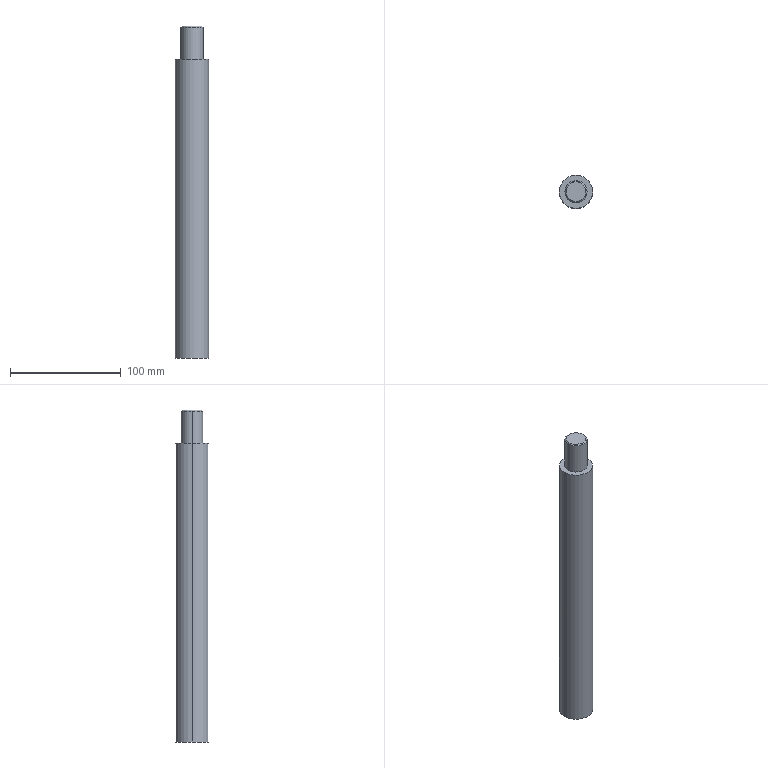Part | STEP file | Telescopic Rod 2 | 1 solid | 9 faces | box 30 x 30 x 300 mm | volume 200246 mm3 | cylinder 4 | plane 3 | cone 2 | commonest cylinder face diameters 20 x2 30 x2
STEP:
#1=CARTESIAN_POINT('',(-15.,0.,270.));
#2=VERTEX_POINT('',#1);
#3=CARTESIAN_POINT('',(15.,0.,270.));
#4=VERTEX_POINT('',#3);
#5=CARTESIAN_POINT('',(0.,0.,270.));
#6=DIRECTION('',(0.,0.,-1.));
#7=DIRECTION('',(-1.,0.,0.));
#8=AXIS2_PLACEMENT_3D('',#5,#6,#7);
#9=CIRCLE('',#8,15.);
#10=EDGE_CURVE('',#2,#4,#9,.T.);
#11=ORIENTED_EDGE('',*,*,#10,.T.);
#12=CARTESIAN_POINT('',(15.,0.,0.));
#13=VERTEX_POINT('',#12);
#14=CARTESIAN_POINT('',(15.,0.,300.));
#15=DIRECTION('',(0.,0.,-1.));
#16=VECTOR('',#15,1000.);
#17=LINE('',#14,#16);
#18=EDGE_CURVE('',#4,#13,#17,.T.);
#19=ORIENTED_EDGE('',*,*,#18,.T.);
#20=CARTESIAN_POINT('',(-15.,0.,0.));
#21=VERTEX_POINT('',#20);
#22=CARTESIAN_POINT('',(0.,0.,0.));
#23=DIRECTION('',(0.,0.,1.));
#24=DIRECTION('',(-1.,0.,0.));
#25=AXIS2_PLACEMENT_3D('',#22,#23,#24);
#26=CIRCLE('',#25,15.);
#27=EDGE_CURVE('',#13,#21,#26,.T.);
#28=ORIENTED_EDGE('',*,*,#27,.T.);
#29=CARTESIAN_POINT('',(-15.,0.,300.));
#30=DIRECTION('',(0.,0.,-1.));
#31=VECTOR('',#30,1000.);
#32=LINE('',#29,#31);
#33=EDGE_CURVE('',#2,#21,#32,.T.);
#34=ORIENTED_EDGE('',*,*,#33,.F.);
#35=EDGE_LOOP('',(#11,#19,#28,#34));
#36=FACE_OUTER_BOUND('',#35,.T.);
#37=CARTESIAN_POINT('',(0.,0.,300.));
#38=DIRECTION('',(0.,0.,-1.));
#39=DIRECTION('',(-1.,0.,0.));
#40=AXIS2_PLACEMENT_3D('',#37,#38,#39);
#41=CYLINDRICAL_SURFACE('',#40,15.);
#42=ADVANCED_FACE('',(#36),#41,.T.);
#43=CARTESIAN_POINT('',(-10.,0.,270.));
#44=VERTEX_POINT('',#43);
#45=CARTESIAN_POINT('',(10.,0.,270.));
#46=VERTEX_POINT('',#45);
#47=CARTESIAN_POINT('',(0.,0.,270.));
#48=DIRECTION('',(0.,0.,-1.));
#49=DIRECTION('',(1.,0.,0.));
#50=AXIS2_PLACEMENT_3D('',#47,#48,#49);
#51=CIRCLE('',#50,10.);
#52=EDGE_CURVE('',#44,#46,#51,.T.);
#53=ORIENTED_EDGE('',*,*,#52,.F.);
#54=CARTESIAN_POINT('',(-10.,0.,299.));
#55=VERTEX_POINT('',#54);
#56=CARTESIAN_POINT('',(-10.,0.,270.));
#57=DIRECTION('',(0.,0.,1.));
#58=VECTOR('',#57,1000.);
#59=LINE('',#56,#58);
#60=EDGE_CURVE('',#44,#55,#59,.T.);
#61=ORIENTED_EDGE('',*,*,#60,.T.);
#62=CARTESIAN_POINT('',(10.,0.,299.));
#63=VERTEX_POINT('',#62);
#64=CARTESIAN_POINT('',(0.,0.,299.));
#65=DIRECTION('',(0.,0.,-1.));
#66=DIRECTION('',(1.,0.,0.));
#67=AXIS2_PLACEMENT_3D('',#64,#65,#66);
#68=CIRCLE('',#67,10.);
#69=EDGE_CURVE('',#55,#63,#68,.T.);
#70=ORIENTED_EDGE('',*,*,#69,.T.);
#71=CARTESIAN_POINT('',(10.,0.,270.));
#72=DIRECTION('',(0.,0.,1.));
#73=VECTOR('',#72,1000.);
#74=LINE('',#71,#73);
#75=EDGE_CURVE('',#46,#63,#74,.T.);
#76=ORIENTED_EDGE('',*,*,#75,.F.);
#77=EDGE_LOOP('',(#53,#61,#70,#76));
#78=FACE_OUTER_BOUND('',#77,.T.);
#79=CARTESIAN_POINT('',(0.,0.,270.));
#80=DIRECTION('',(0.,0.,1.));
#81=DIRECTION('',(1.,0.,0.));
#82=AXIS2_PLACEMENT_3D('',#79,#80,#81);
#83=CYLINDRICAL_SURFACE('',#82,10.);
#84=ADVANCED_FACE('',(#78),#83,.T.);
#85=CARTESIAN_POINT('',(-9.,0.,300.));
#86=VERTEX_POINT('',#85);
#87=CARTESIAN_POINT('',(9.,0.,300.));
#88=VERTEX_POINT('',#87);
#89=CARTESIAN_POINT('',(0.,0.,300.));
#90=DIRECTION('',(0.,0.,-1.));
#91=DIRECTION('',(-1.,0.,0.));
#92=AXIS2_PLACEMENT_3D('',#89,#90,#91);
#93=CIRCLE('',#92,9.);
#94=EDGE_CURVE('',#86,#88,#93,.T.);
#95=ORIENTED_EDGE('',*,*,#94,.T.);
#96=CARTESIAN_POINT('',(10.,0.,299.));
#97=DIRECTION('',(0.7071,0.,-0.7071));
#98=VECTOR('',#97,1000.);
#99=LINE('',#96,#98);
#100=EDGE_CURVE('',#88,#63,#99,.T.);
#101=ORIENTED_EDGE('',*,*,#100,.T.);
#102=ORIENTED_EDGE('',*,*,#69,.F.);
#103=CARTESIAN_POINT('',(-10.,0.,299.));
#104=DIRECTION('',(-0.7071,0.,-0.7071));
#105=VECTOR('',#104,1000.);
#106=LINE('',#103,#105);
#107=EDGE_CURVE('',#86,#55,#106,.T.);
#108=ORIENTED_EDGE('',*,*,#107,.F.);
#109=EDGE_LOOP('',(#95,#101,#102,#108));
#110=FACE_OUTER_BOUND('',#109,.T.);
#111=CARTESIAN_POINT('',(0.,0.,299.));
#112=DIRECTION('',(0.,0.,-1.));
#113=DIRECTION('',(-1.,0.,0.));
#114=AXIS2_PLACEMENT_3D('',#111,#112,#113);
#115=CONICAL_SURFACE('',#114,10.,0.7854);
#116=ADVANCED_FACE('',(#110),#115,.T.);
#117=ORIENTED_EDGE('',*,*,#18,.F.);
#118=CARTESIAN_POINT('',(0.,0.,270.));
#119=DIRECTION('',(0.,0.,-1.));
#120=DIRECTION('',(-1.,0.,0.));
#121=AXIS2_PLACEMENT_3D('',#118,#119,#120);
#122=CIRCLE('',#121,15.);
#123=EDGE_CURVE('',#4,#2,#122,.T.);
#124=ORIENTED_EDGE('',*,*,#123,.T.);
#125=ORIENTED_EDGE('',*,*,#33,.T.);
#126=CARTESIAN_POINT('',(0.,0.,0.));
#127=DIRECTION('',(0.,0.,1.));
#128=DIRECTION('',(-1.,0.,0.));
#129=AXIS2_PLACEMENT_3D('',#126,#127,#128);
#130=CIRCLE('',#129,15.);
#131=EDGE_CURVE('',#21,#13,#130,.T.);
#132=ORIENTED_EDGE('',*,*,#131,.T.);
#133=EDGE_LOOP('',(#117,#124,#125,#132));
#134=FACE_OUTER_BOUND('',#133,.T.);
#135=CARTESIAN_POINT('',(0.,0.,300.));
#136=DIRECTION('',(0.,0.,-1.));
#137=DIRECTION('',(-1.,0.,0.));
#138=AXIS2_PLACEMENT_3D('',#135,#136,#137);
#139=CYLINDRICAL_SURFACE('',#138,15.);
#140=ADVANCED_FACE('',(#134),#139,.T.);
#141=ORIENTED_EDGE('',*,*,#131,.F.);
#142=ORIENTED_EDGE('',*,*,#27,.F.);
#143=EDGE_LOOP('',(#141,#142));
#144=FACE_OUTER_BOUND('',#143,.T.);
#145=CARTESIAN_POINT('',(0.,0.,0.));
#146=DIRECTION('',(0.,0.,1.));
#147=DIRECTION('',(1.,0.,0.));
#148=AXIS2_PLACEMENT_3D('',#145,#146,#147);
#149=PLANE('',#148);
#150=ADVANCED_FACE('',(#144),#149,.F.);
#151=ORIENTED_EDGE('',*,*,#10,.F.);
#152=ORIENTED_EDGE('',*,*,#123,.F.);
#153=EDGE_LOOP('',(#151,#152));
#154=FACE_OUTER_BOUND('',#153,.T.);
#155=CARTESIAN_POINT('',(0.,0.,270.));
#156=DIRECTION('',(0.,0.,-1.));
#157=DIRECTION('',(1.,0.,0.));
#158=AXIS2_PLACEMENT_3D('',#155,#156,#157);
#159=CIRCLE('',#158,10.);
#160=EDGE_CURVE('',#46,#44,#159,.T.);
#161=ORIENTED_EDGE('',*,*,#160,.T.);
#162=ORIENTED_EDGE('',*,*,#52,.T.);
#163=EDGE_LOOP('',(#161,#162));
#164=FACE_BOUND('',#163,.T.);
#165=CARTESIAN_POINT('',(0.,0.,270.));
#166=DIRECTION('',(0.,0.,1.));
#167=DIRECTION('',(1.,0.,0.));
#168=AXIS2_PLACEMENT_3D('',#165,#166,#167);
#169=PLANE('',#168);
#170=ADVANCED_FACE('',(#154,#164),#169,.T.);
#171=ORIENTED_EDGE('',*,*,#60,.F.);
#172=ORIENTED_EDGE('',*,*,#160,.F.);
#173=ORIENTED_EDGE('',*,*,#75,.T.);
#174=CARTESIAN_POINT('',(0.,0.,299.));
#175=DIRECTION('',(0.,0.,-1.));
#176=DIRECTION('',(1.,0.,0.));
#177=AXIS2_PLACEMENT_3D('',#174,#175,#176);
#178=CIRCLE('',#177,10.);
#179=EDGE_CURVE('',#63,#55,#178,.T.);
#180=ORIENTED_EDGE('',*,*,#179,.T.);
#181=EDGE_LOOP('',(#171,#172,#173,#180));
#182=FACE_OUTER_BOUND('',#181,.T.);
#183=CARTESIAN_POINT('',(0.,0.,270.));
#184=DIRECTION('',(0.,0.,1.));
#185=DIRECTION('',(1.,0.,0.));
#186=AXIS2_PLACEMENT_3D('',#183,#184,#185);
#187=CYLINDRICAL_SURFACE('',#186,10.);
#188=ADVANCED_FACE('',(#182),#187,.T.);
#189=ORIENTED_EDGE('',*,*,#100,.F.);
#190=CARTESIAN_POINT('',(0.,0.,300.));
#191=DIRECTION('',(0.,0.,-1.));
#192=DIRECTION('',(-1.,0.,0.));
#193=AXIS2_PLACEMENT_3D('',#190,#191,#192);
#194=CIRCLE('',#193,9.);
#195=EDGE_CURVE('',#88,#86,#194,.T.);
#196=ORIENTED_EDGE('',*,*,#195,.T.);
#197=ORIENTED_EDGE('',*,*,#107,.T.);
#198=ORIENTED_EDGE('',*,*,#179,.F.);
#199=EDGE_LOOP('',(#189,#196,#197,#198));
#200=FACE_OUTER_BOUND('',#199,.T.);
#201=CARTESIAN_POINT('',(0.,0.,299.));
#202=DIRECTION('',(0.,0.,-1.));
#203=DIRECTION('',(-1.,0.,0.));
#204=AXIS2_PLACEMENT_3D('',#201,#202,#203);
#205=CONICAL_SURFACE('',#204,10.,0.7854);
#206=ADVANCED_FACE('',(#200),#205,.T.);
#207=ORIENTED_EDGE('',*,*,#94,.F.);
#208=ORIENTED_EDGE('',*,*,#195,.F.);
#209=EDGE_LOOP('',(#207,#208));
#210=FACE_OUTER_BOUND('',#209,.T.);
#211=CARTESIAN_POINT('',(0.,0.,300.));
#212=DIRECTION('',(0.,0.,1.));
#213=DIRECTION('',(1.,0.,0.));
#214=AXIS2_PLACEMENT_3D('',#211,#212,#213);
#215=PLANE('',#214);
#216=ADVANCED_FACE('',(#210),#215,.T.);
#217=CLOSED_SHELL('',(#42,#84,#116,#140,#150,#170,#188,#206,#216));
#218=MANIFOLD_SOLID_BREP('',#217);
#219=CARTESIAN_POINT('',(0.,0.,0.));
#220=DIRECTION('',(0.,0.,1.));
#221=DIRECTION('',(1.,0.,0.));
#222=AXIS2_PLACEMENT_3D('',#219,#220,#221);
#223=(LENGTH_UNIT()NAMED_UNIT(*)SI_UNIT(.MILLI.,.METRE.));
#224=UNCERTAINTY_MEASURE_WITH_UNIT(LENGTH_MEASURE(0.00001),#223,'','');
#225=(NAMED_UNIT(*)PLANE_ANGLE_UNIT()SI_UNIT($,.RADIAN.));
#226=(NAMED_UNIT(*)SI_UNIT($,.STERADIAN.)SOLID_ANGLE_UNIT());
#227=(GEOMETRIC_REPRESENTATION_CONTEXT(3)GLOBAL_UNCERTAINTY_ASSIGNED_CONTEXT((#224))GLOBAL_UNIT_ASSIGNED_CONTEXT((#223,#225,#226))REPRESENTATION_CONTEXT('',''));
#228=ADVANCED_BREP_SHAPE_REPRESENTATION('',(#218,#222),#227);